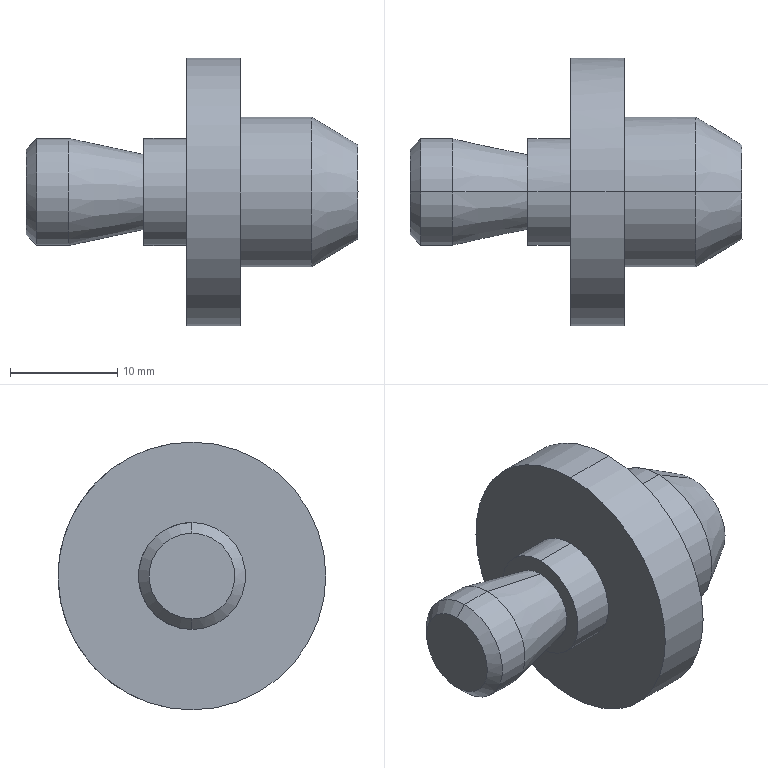Part | STEP file | Positioning_id1706_x_t | 1 solid | 19 faces | box 31 x 25 x 25 mm | volume 4946 mm3 | cylinder 8 | cone 6 | plane 5 | commonest cylinder face diameters 10 x4 14 x2 25 x2
STEP:
#1=CARTESIAN_POINT('',(0.,0.,0.));
#2=DIRECTION('',(0.,0.,1.));
#3=DIRECTION('',(1.,0.,0.));
#4=AXIS2_PLACEMENT_3D('',#1,#2,#3);
#5=CARTESIAN_POINT('',(-652.333,523.,129.997));
#6=VERTEX_POINT('',#5);
#7=CARTESIAN_POINT('',(-648.,523.,127.397));
#8=VERTEX_POINT('',#7);
#9=CARTESIAN_POINT('',(-648.,523.,127.397));
#10=DIRECTION('',(0.8575,0.,-0.5145));
#11=VECTOR('',#10,1.);
#12=LINE('',#9,#11);
#13=CARTESIAN_POINT('',(-654.,523.,122.997));
#14=DIRECTION('',(-1.,0.,0.));
#15=DIRECTION('',(0.,0.,1.));
#16=AXIS2_PLACEMENT_3D('',#13,#14,#15);
#17=CONICAL_SURFACE('',#16,8.,0.5404);
#18=CARTESIAN_POINT('',(0.,-6.));
#19=DIRECTION('',(0.,-1.));
#20=VECTOR('',#19,1.);
#21=LINE('',#18,#20);
#22=(GEOMETRIC_REPRESENTATION_CONTEXT(2)PARAMETRIC_REPRESENTATION_CONTEXT()REPRESENTATION_CONTEXT('',''));
#23=DEFINITIONAL_REPRESENTATION('',(#21),#22);
#24=PCURVE('',#17,#23);
#25=CARTESIAN_POINT('',(-654.,523.,122.997));
#26=DIRECTION('',(-1.,0.,0.));
#27=DIRECTION('',(0.,0.,1.));
#28=AXIS2_PLACEMENT_3D('',#25,#26,#27);
#29=CONICAL_SURFACE('',#28,8.,0.5404);
#30=CARTESIAN_POINT('',(6.283,-6.));
#31=DIRECTION('',(0.,-1.));
#32=VECTOR('',#31,1.);
#33=LINE('',#30,#32);
#34=(GEOMETRIC_REPRESENTATION_CONTEXT(2)PARAMETRIC_REPRESENTATION_CONTEXT()REPRESENTATION_CONTEXT('',''));
#35=DEFINITIONAL_REPRESENTATION('',(#33),#34);
#36=PCURVE('',#29,#35);
#37=SURFACE_CURVE('',#12,(#24,#36),.PCURVE_S1.);
#38=EDGE_CURVE('',#6,#8,#37,.T.);
#39=ORIENTED_EDGE('',*,*,#38,.T.);
#40=CARTESIAN_POINT('',(-648.,523.,118.597));
#41=VERTEX_POINT('',#40);
#42=CARTESIAN_POINT('',(-648.,523.,122.997));
#43=DIRECTION('',(-1.,0.,0.));
#44=DIRECTION('',(0.,0.,1.));
#45=AXIS2_PLACEMENT_3D('',#42,#43,#44);
#46=CIRCLE('',#45,4.4);
#47=CARTESIAN_POINT('',(0.,-6.));
#48=DIRECTION('',(1.,0.));
#49=VECTOR('',#48,1.);
#50=LINE('',#47,#49);
#51=(GEOMETRIC_REPRESENTATION_CONTEXT(2)PARAMETRIC_REPRESENTATION_CONTEXT()REPRESENTATION_CONTEXT('',''));
#52=DEFINITIONAL_REPRESENTATION('',(#50),#51);
#53=PCURVE('',#17,#52);
#54=CARTESIAN_POINT('',(-648.,523.,122.997));
#55=DIRECTION('',(1.,0.,0.));
#56=DIRECTION('',(0.,0.,1.));
#57=AXIS2_PLACEMENT_3D('',#54,#55,#56);
#58=PLANE('',#57);
#59=CARTESIAN_POINT('',(4.4,0.));
#60=CARTESIAN_POINT('',(4.4,-7.621));
#61=CARTESIAN_POINT('',(-2.2,-3.811));
#62=CARTESIAN_POINT('',(-8.8,0.));
#63=CARTESIAN_POINT('',(-2.2,3.811));
#64=CARTESIAN_POINT('',(4.4,7.621));
#65=CARTESIAN_POINT('',(4.4,0.));
#66=(BOUNDED_CURVE()B_SPLINE_CURVE(2,(#59,#60,#61,#62,#63,#64,#65),.UNSPECIFIED.,.T.,.F.)B_SPLINE_CURVE_WITH_KNOTS((1,2,2,2,2,1),(-2.094,0.,2.094,4.189,6.283,8.378),.UNSPECIFIED.)CURVE()GEOMETRIC_REPRESENTATION_ITEM()RATIONAL_B_SPLINE_CURVE((1.,0.5,1.,0.5,1.,0.5,1.))REPRESENTATION_ITEM(''));
#67=(GEOMETRIC_REPRESENTATION_CONTEXT(2)PARAMETRIC_REPRESENTATION_CONTEXT()REPRESENTATION_CONTEXT('',''));
#68=DEFINITIONAL_REPRESENTATION('',(#66),#67);
#69=PCURVE('',#58,#68);
#70=SURFACE_CURVE('',#46,(#53,#69),.PCURVE_S1.);
#71=EDGE_CURVE('',#8,#41,#70,.T.);
#72=ORIENTED_EDGE('',*,*,#71,.T.);
#73=CARTESIAN_POINT('',(-652.333,523.,115.997));
#74=VERTEX_POINT('',#73);
#75=CARTESIAN_POINT('',(-648.,523.,118.597));
#76=DIRECTION('',(-0.8575,0.,-0.5145));
#77=VECTOR('',#76,1.);
#78=LINE('',#75,#77);
#79=CARTESIAN_POINT('',(3.142,-6.));
#80=DIRECTION('',(0.,1.));
#81=VECTOR('',#80,1.);
#82=LINE('',#79,#81);
#83=(GEOMETRIC_REPRESENTATION_CONTEXT(2)PARAMETRIC_REPRESENTATION_CONTEXT()REPRESENTATION_CONTEXT('',''));
#84=DEFINITIONAL_REPRESENTATION('',(#82),#83);
#85=PCURVE('',#17,#84);
#86=CARTESIAN_POINT('',(3.142,-6.));
#87=DIRECTION('',(0.,1.));
#88=VECTOR('',#87,1.);
#89=LINE('',#86,#88);
#90=(GEOMETRIC_REPRESENTATION_CONTEXT(2)PARAMETRIC_REPRESENTATION_CONTEXT()REPRESENTATION_CONTEXT('',''));
#91=DEFINITIONAL_REPRESENTATION('',(#89),#90);
#92=PCURVE('',#29,#91);
#93=SURFACE_CURVE('',#78,(#85,#92),.PCURVE_S1.);
#94=EDGE_CURVE('',#41,#74,#93,.T.);
#95=ORIENTED_EDGE('',*,*,#94,.T.);
#96=CARTESIAN_POINT('',(-652.333,523.,122.997));
#97=DIRECTION('',(1.,0.,0.));
#98=DIRECTION('',(0.,0.,-1.));
#99=AXIS2_PLACEMENT_3D('',#96,#97,#98);
#100=CIRCLE('',#99,7.);
#101=CARTESIAN_POINT('',(3.142,-1.667));
#102=DIRECTION('',(-1.,0.));
#103=VECTOR('',#102,1.);
#104=LINE('',#101,#103);
#105=(GEOMETRIC_REPRESENTATION_CONTEXT(2)PARAMETRIC_REPRESENTATION_CONTEXT()REPRESENTATION_CONTEXT('',''));
#106=DEFINITIONAL_REPRESENTATION('',(#104),#105);
#107=PCURVE('',#17,#106);
#108=CARTESIAN_POINT('',(-659.,523.,122.997));
#109=DIRECTION('',(-1.,0.,0.));
#110=DIRECTION('',(0.,0.,1.));
#111=AXIS2_PLACEMENT_3D('',#108,#109,#110);
#112=CYLINDRICAL_SURFACE('',#111,7.);
#113=CARTESIAN_POINT('',(3.142,-6.667));
#114=DIRECTION('',(-1.,0.));
#115=VECTOR('',#114,1.);
#116=LINE('',#113,#115);
#117=(GEOMETRIC_REPRESENTATION_CONTEXT(2)PARAMETRIC_REPRESENTATION_CONTEXT()REPRESENTATION_CONTEXT('',''));
#118=DEFINITIONAL_REPRESENTATION('',(#116),#117);
#119=PCURVE('',#112,#118);
#120=SURFACE_CURVE('',#100,(#107,#119),.PCURVE_S1.);
#121=EDGE_CURVE('',#74,#6,#120,.T.);
#122=ORIENTED_EDGE('',*,*,#121,.T.);
#123=EDGE_LOOP('',(#39,#72,#95,#122));
#124=FACE_BOUND('',#123,.T.);
#125=ADVANCED_FACE('',(#124),#17,.T.);
#126=CARTESIAN_POINT('',(-659.,523.,129.997));
#127=VERTEX_POINT('',#126);
#128=CARTESIAN_POINT('',(-659.,523.,129.997));
#129=DIRECTION('',(1.,0.,0.));
#130=VECTOR('',#129,1.);
#131=LINE('',#128,#130);
#132=CARTESIAN_POINT('',(-659.,523.,122.997));
#133=DIRECTION('',(-1.,0.,0.));
#134=DIRECTION('',(0.,0.,1.));
#135=AXIS2_PLACEMENT_3D('',#132,#133,#134);
#136=CYLINDRICAL_SURFACE('',#135,7.);
#137=CARTESIAN_POINT('',(6.283,0.));
#138=DIRECTION('',(0.,-1.));
#139=VECTOR('',#138,1.);
#140=LINE('',#137,#139);
#141=(GEOMETRIC_REPRESENTATION_CONTEXT(2)PARAMETRIC_REPRESENTATION_CONTEXT()REPRESENTATION_CONTEXT('',''));
#142=DEFINITIONAL_REPRESENTATION('',(#140),#141);
#143=PCURVE('',#136,#142);
#144=CARTESIAN_POINT('',(0.,0.));
#145=DIRECTION('',(0.,-1.));
#146=VECTOR('',#145,1.);
#147=LINE('',#144,#146);
#148=(GEOMETRIC_REPRESENTATION_CONTEXT(2)PARAMETRIC_REPRESENTATION_CONTEXT()REPRESENTATION_CONTEXT('',''));
#149=DEFINITIONAL_REPRESENTATION('',(#147),#148);
#150=PCURVE('',#112,#149);
#151=SURFACE_CURVE('',#131,(#143,#150),.PCURVE_S1.);
#152=EDGE_CURVE('',#127,#6,#151,.T.);
#153=ORIENTED_EDGE('',*,*,#152,.F.);
#154=CARTESIAN_POINT('',(-659.,523.,115.997));
#155=VERTEX_POINT('',#154);
#156=CARTESIAN_POINT('',(-659.,523.,122.997));
#157=DIRECTION('',(-1.,0.,0.));
#158=DIRECTION('',(0.,0.,1.));
#159=AXIS2_PLACEMENT_3D('',#156,#157,#158);
#160=CIRCLE('',#159,7.);
#161=CARTESIAN_POINT('',(0.,0.));
#162=DIRECTION('',(1.,0.));
#163=VECTOR('',#162,1.);
#164=LINE('',#161,#163);
#165=(GEOMETRIC_REPRESENTATION_CONTEXT(2)PARAMETRIC_REPRESENTATION_CONTEXT()REPRESENTATION_CONTEXT('',''));
#166=DEFINITIONAL_REPRESENTATION('',(#164),#165);
#167=PCURVE('',#136,#166);
#168=CARTESIAN_POINT('',(-659.,523.,122.997));
#169=DIRECTION('',(1.,0.,0.));
#170=DIRECTION('',(0.,0.,1.));
#171=AXIS2_PLACEMENT_3D('',#168,#169,#170);
#172=PLANE('',#171);
#173=CARTESIAN_POINT('',(7.,0.));
#174=CARTESIAN_POINT('',(7.,-12.124));
#175=CARTESIAN_POINT('',(-3.5,-6.062));
#176=CARTESIAN_POINT('',(-14.,0.));
#177=CARTESIAN_POINT('',(-3.5,6.062));
#178=CARTESIAN_POINT('',(7.,12.124));
#179=CARTESIAN_POINT('',(7.,0.));
#180=(BOUNDED_CURVE()B_SPLINE_CURVE(2,(#173,#174,#175,#176,#177,#178,#179),.UNSPECIFIED.,.T.,.F.)B_SPLINE_CURVE_WITH_KNOTS((1,2,2,2,2,1),(-2.094,0.,2.094,4.189,6.283,8.378),.UNSPECIFIED.)CURVE()GEOMETRIC_REPRESENTATION_ITEM()RATIONAL_B_SPLINE_CURVE((1.,0.5,1.,0.5,1.,0.5,1.))REPRESENTATION_ITEM(''));
#181=(GEOMETRIC_REPRESENTATION_CONTEXT(2)PARAMETRIC_REPRESENTATION_CONTEXT()REPRESENTATION_CONTEXT('',''));
#182=DEFINITIONAL_REPRESENTATION('',(#180),#181);
#183=PCURVE('',#172,#182);
#184=SURFACE_CURVE('',#160,(#167,#183),.PCURVE_S1.);
#185=EDGE_CURVE('',#155,#127,#184,.T.);
#186=ORIENTED_EDGE('',*,*,#185,.F.);
#187=CARTESIAN_POINT('',(-659.,523.,115.997));
#188=DIRECTION('',(-1.,0.,0.));
#189=VECTOR('',#188,1.);
#190=LINE('',#187,#189);
#191=CARTESIAN_POINT('',(3.142,0.));
#192=DIRECTION('',(0.,1.));
#193=VECTOR('',#192,1.);
#194=LINE('',#191,#193);
#195=(GEOMETRIC_REPRESENTATION_CONTEXT(2)PARAMETRIC_REPRESENTATION_CONTEXT()REPRESENTATION_CONTEXT('',''));
#196=DEFINITIONAL_REPRESENTATION('',(#194),#195);
#197=PCURVE('',#136,#196);
#198=CARTESIAN_POINT('',(3.142,0.));
#199=DIRECTION('',(0.,1.));
#200=VECTOR('',#199,1.);
#201=LINE('',#198,#200);
#202=(GEOMETRIC_REPRESENTATION_CONTEXT(2)PARAMETRIC_REPRESENTATION_CONTEXT()REPRESENTATION_CONTEXT('',''));
#203=DEFINITIONAL_REPRESENTATION('',(#201),#202);
#204=PCURVE('',#112,#203);
#205=SURFACE_CURVE('',#190,(#197,#204),.PCURVE_S1.);
#206=EDGE_CURVE('',#74,#155,#205,.T.);
#207=ORIENTED_EDGE('',*,*,#206,.F.);
#208=CARTESIAN_POINT('',(-652.333,523.,122.997));
#209=DIRECTION('',(1.,0.,0.));
#210=DIRECTION('',(0.,0.,1.));
#211=AXIS2_PLACEMENT_3D('',#208,#209,#210);
#212=CIRCLE('',#211,7.);
#213=CARTESIAN_POINT('',(6.283,-6.667));
#214=DIRECTION('',(-1.,0.));
#215=VECTOR('',#214,1.);
#216=LINE('',#213,#215);
#217=(GEOMETRIC_REPRESENTATION_CONTEXT(2)PARAMETRIC_REPRESENTATION_CONTEXT()REPRESENTATION_CONTEXT('',''));
#218=DEFINITIONAL_REPRESENTATION('',(#216),#217);
#219=PCURVE('',#136,#218);
#220=CARTESIAN_POINT('',(6.283,-1.667));
#221=DIRECTION('',(-1.,0.));
#222=VECTOR('',#221,1.);
#223=LINE('',#220,#222);
#224=(GEOMETRIC_REPRESENTATION_CONTEXT(2)PARAMETRIC_REPRESENTATION_CONTEXT()REPRESENTATION_CONTEXT('',''));
#225=DEFINITIONAL_REPRESENTATION('',(#223),#224);
#226=PCURVE('',#29,#225);
#227=SURFACE_CURVE('',#212,(#219,#226),.PCURVE_S1.);
#228=EDGE_CURVE('',#6,#74,#227,.T.);
#229=ORIENTED_EDGE('',*,*,#228,.F.);
#230=EDGE_LOOP('',(#153,#186,#207,#229));
#231=FACE_BOUND('',#230,.T.);
#232=ADVANCED_FACE('',(#231),#136,.T.);
#233=CARTESIAN_POINT('',(-648.,523.,118.597));
#234=CARTESIAN_POINT('',(-648.,518.6,118.597));
#235=CARTESIAN_POINT('',(-648.,516.4,122.997));
#236=CARTESIAN_POINT('',(-648.,518.6,127.397));
#237=CARTESIAN_POINT('',(-648.,523.,127.397));
#238=(BOUNDED_CURVE()B_SPLINE_CURVE(4,(#233,#234,#235,#236,#237),.UNSPECIFIED.,.F.,.F.)B_SPLINE_CURVE_WITH_KNOTS((5,5),(0.,1.),.PIECEWISE_BEZIER_KNOTS.)CURVE()GEOMETRIC_REPRESENTATION_ITEM()RATIONAL_B_SPLINE_CURVE((1.,0.7071,0.6667,0.7071,1.))REPRESENTATION_ITEM(''));
#239=CARTESIAN_POINT('',(-4.4,0.));
#240=CARTESIAN_POINT('',(-4.4,4.4));
#241=CARTESIAN_POINT('',(0.,6.6));
#242=CARTESIAN_POINT('',(4.4,4.4));
#243=CARTESIAN_POINT('',(4.4,0.));
#244=(BOUNDED_CURVE()B_SPLINE_CURVE(4,(#239,#240,#241,#242,#243),.UNSPECIFIED.,.F.,.F.)B_SPLINE_CURVE_WITH_KNOTS((5,5),(0.,1.),.PIECEWISE_BEZIER_KNOTS.)CURVE()GEOMETRIC_REPRESENTATION_ITEM()RATIONAL_B_SPLINE_CURVE((1.,0.7071,0.6667,0.7071,1.))REPRESENTATION_ITEM(''));
#245=(GEOMETRIC_REPRESENTATION_CONTEXT(2)PARAMETRIC_REPRESENTATION_CONTEXT()REPRESENTATION_CONTEXT('',''));
#246=DEFINITIONAL_REPRESENTATION('',(#244),#245);
#247=PCURVE('',#58,#246);
#248=CARTESIAN_POINT('',(3.142,-6.));
#249=CARTESIAN_POINT('',(3.184,-6.));
#250=CARTESIAN_POINT('',(3.271,-6.));
#251=CARTESIAN_POINT('',(3.405,-6.));
#252=CARTESIAN_POINT('',(3.542,-6.));
#253=CARTESIAN_POINT('',(3.681,-6.));
#254=CARTESIAN_POINT('',(3.823,-6.));
#255=CARTESIAN_POINT('',(3.968,-6.));
#256=CARTESIAN_POINT('',(4.114,-6.));
#257=CARTESIAN_POINT('',(4.262,-6.));
#258=CARTESIAN_POINT('',(4.412,-6.));
#259=CARTESIAN_POINT('',(4.562,-6.));
#260=CARTESIAN_POINT('',(4.712,-6.));
#261=CARTESIAN_POINT('',(4.863,-6.));
#262=CARTESIAN_POINT('',(5.013,-6.));
#263=CARTESIAN_POINT('',(5.163,-6.));
#264=CARTESIAN_POINT('',(5.311,-6.));
#265=CARTESIAN_POINT('',(5.457,-6.));
#266=CARTESIAN_POINT('',(5.602,-6.));
#267=CARTESIAN_POINT('',(5.744,-6.));
#268=CARTESIAN_POINT('',(5.883,-6.));
#269=CARTESIAN_POINT('',(6.02,-6.));
#270=CARTESIAN_POINT('',(6.153,-6.));
#271=CARTESIAN_POINT('',(6.24,-6.));
#272=CARTESIAN_POINT('',(6.283,-6.));
#273=B_SPLINE_CURVE_WITH_KNOTS('',3,(#248,#249,#250,#251,#252,#253,#254,#255,#256,#257,#258,#259,#260,#261,#262,#263,#264,#265,#266,#267,#268,#269,#270,#271,#272),.UNSPECIFIED.,.F.,.F.,(4,1,1,1,1,1,1,1,1,1,1,1,1,1,1,1,1,1,1,1,1,1,4),(0.,0.04545,0.09091,0.1364,0.1818,0.2273,0.2727,0.3182,0.3636,0.4091,0.4545,0.5,0.5455,0.5909,0.6364,0.6818,0.7273,0.7727,0.8182,0.8636,0.9091,0.9545,1.),.QUASI_UNIFORM_KNOTS.);
#274=(GEOMETRIC_REPRESENTATION_CONTEXT(2)PARAMETRIC_REPRESENTATION_CONTEXT()REPRESENTATION_CONTEXT('',''));
#275=DEFINITIONAL_REPRESENTATION('',(#273),#274);
#276=PCURVE('',#29,#275);
#277=SURFACE_CURVE('',#238,(#247,#276),.PCURVE_S1.);
#278=EDGE_CURVE('',#41,#8,#277,.T.);
#279=ORIENTED_EDGE('',*,*,#278,.F.);
#280=ORIENTED_EDGE('',*,*,#71,.F.);
#281=EDGE_LOOP('',(#279,#280));
#282=FACE_BOUND('',#281,.T.);
#283=ADVANCED_FACE('',(#282),#58,.T.);
#284=CARTESIAN_POINT('',(-668.,523.,119.497));
#285=VERTEX_POINT('',#284);
#286=CARTESIAN_POINT('',(-668.,523.,126.497));
#287=VERTEX_POINT('',#286);
#288=CARTESIAN_POINT('',(-668.,523.,122.997));
#289=DIRECTION('',(-1.,0.,0.));
#290=DIRECTION('',(0.,0.,-1.));
#291=AXIS2_PLACEMENT_3D('',#288,#289,#290);
#292=CIRCLE('',#291,3.5);
#293=CARTESIAN_POINT('',(-668.,523.,122.997));
#294=DIRECTION('',(1.,0.,0.));
#295=DIRECTION('',(0.,0.,1.));
#296=AXIS2_PLACEMENT_3D('',#293,#294,#295);
#297=PLANE('',#296);
#298=CARTESIAN_POINT('',(-3.5,0.));
#299=CARTESIAN_POINT('',(-3.5,6.062));
#300=CARTESIAN_POINT('',(1.75,3.031));
#301=CARTESIAN_POINT('',(7.,0.));
#302=CARTESIAN_POINT('',(1.75,-3.031));
#303=CARTESIAN_POINT('',(-3.5,-6.062));
#304=CARTESIAN_POINT('',(-3.5,0.));
#305=(BOUNDED_CURVE()B_SPLINE_CURVE(2,(#298,#299,#300,#301,#302,#303,#304),.UNSPECIFIED.,.T.,.F.)B_SPLINE_CURVE_WITH_KNOTS((1,2,2,2,2,1),(-2.094,0.,2.094,4.189,6.283,8.378),.UNSPECIFIED.)CURVE()GEOMETRIC_REPRESENTATION_ITEM()RATIONAL_B_SPLINE_CURVE((1.,0.5,1.,0.5,1.,0.5,1.))REPRESENTATION_ITEM(''));
#306=(GEOMETRIC_REPRESENTATION_CONTEXT(2)PARAMETRIC_REPRESENTATION_CONTEXT()REPRESENTATION_CONTEXT('',''));
#307=DEFINITIONAL_REPRESENTATION('',(#305),#306);
#308=PCURVE('',#297,#307);
#309=CARTESIAN_POINT('',(-675.,523.,122.997));
#310=DIRECTION('',(-1.,0.,0.));
#311=DIRECTION('',(0.,0.,1.));
#312=AXIS2_PLACEMENT_3D('',#309,#310,#311);
#313=CONICAL_SURFACE('',#312,5.,0.2111);
#314=CARTESIAN_POINT('',(3.142,-7.));
#315=DIRECTION('',(1.,0.));
#316=VECTOR('',#315,1.);
#317=LINE('',#314,#316);
#318=(GEOMETRIC_REPRESENTATION_CONTEXT(2)PARAMETRIC_REPRESENTATION_CONTEXT()REPRESENTATION_CONTEXT('',''));
#319=DEFINITIONAL_REPRESENTATION('',(#317),#318);
#320=PCURVE('',#313,#319);
#321=SURFACE_CURVE('',#292,(#308,#320),.PCURVE_S1.);
#322=EDGE_CURVE('',#285,#287,#321,.T.);
#323=ORIENTED_EDGE('',*,*,#322,.F.);
#324=CARTESIAN_POINT('',(-668.,523.,122.997));
#325=DIRECTION('',(-1.,0.,0.));
#326=DIRECTION('',(0.,0.,1.));
#327=AXIS2_PLACEMENT_3D('',#324,#325,#326);
#328=CIRCLE('',#327,3.5);
#329=CARTESIAN_POINT('',(3.5,0.));
#330=CARTESIAN_POINT('',(3.5,-6.062));
#331=CARTESIAN_POINT('',(-1.75,-3.031));
#332=CARTESIAN_POINT('',(-7.,0.));
#333=CARTESIAN_POINT('',(-1.75,3.031));
#334=CARTESIAN_POINT('',(3.5,6.062));
#335=CARTESIAN_POINT('',(3.5,0.));
#336=(BOUNDED_CURVE()B_SPLINE_CURVE(2,(#329,#330,#331,#332,#333,#334,#335),.UNSPECIFIED.,.T.,.F.)B_SPLINE_CURVE_WITH_KNOTS((1,2,2,2,2,1),(-2.094,0.,2.094,4.189,6.283,8.378),.UNSPECIFIED.)CURVE()GEOMETRIC_REPRESENTATION_ITEM()RATIONAL_B_SPLINE_CURVE((1.,0.5,1.,0.5,1.,0.5,1.))REPRESENTATION_ITEM(''));
#337=(GEOMETRIC_REPRESENTATION_CONTEXT(2)PARAMETRIC_REPRESENTATION_CONTEXT()REPRESENTATION_CONTEXT('',''));
#338=DEFINITIONAL_REPRESENTATION('',(#336),#337);
#339=PCURVE('',#297,#338);
#340=CARTESIAN_POINT('',(-675.,523.,122.997));
#341=DIRECTION('',(-1.,0.,0.));
#342=DIRECTION('',(0.,0.,1.));
#343=AXIS2_PLACEMENT_3D('',#340,#341,#342);
#344=CONICAL_SURFACE('',#343,5.,0.2111);
#345=CARTESIAN_POINT('',(0.,-7.));
#346=DIRECTION('',(1.,0.));
#347=VECTOR('',#346,1.);
#348=LINE('',#345,#347);
#349=(GEOMETRIC_REPRESENTATION_CONTEXT(2)PARAMETRIC_REPRESENTATION_CONTEXT()REPRESENTATION_CONTEXT('',''));
#350=DEFINITIONAL_REPRESENTATION('',(#348),#349);
#351=PCURVE('',#344,#350);
#352=SURFACE_CURVE('',#328,(#339,#351),.PCURVE_S1.);
#353=EDGE_CURVE('',#287,#285,#352,.T.);
#354=ORIENTED_EDGE('',*,*,#353,.F.);
#355=EDGE_LOOP('',(#323,#354));
#356=FACE_BOUND('',#355,.T.);
#357=CARTESIAN_POINT('',(-668.,523.,117.997));
#358=VERTEX_POINT('',#357);
#359=CARTESIAN_POINT('',(-668.,523.,127.997));
#360=VERTEX_POINT('',#359);
#361=CARTESIAN_POINT('',(-668.,523.,122.997));
#362=DIRECTION('',(1.,0.,0.));
#363=DIRECTION('',(0.,0.,-1.));
#364=AXIS2_PLACEMENT_3D('',#361,#362,#363);
#365=CIRCLE('',#364,5.);
#366=CARTESIAN_POINT('',(0.,0.));
#367=DIRECTION('',(-1.,0.));
#368=AXIS2_PLACEMENT_2D('',#366,#367);
#369=CIRCLE('',#368,5.);
#370=(GEOMETRIC_REPRESENTATION_CONTEXT(2)PARAMETRIC_REPRESENTATION_CONTEXT()REPRESENTATION_CONTEXT('',''));
#371=DEFINITIONAL_REPRESENTATION('',(#369),#370);
#372=PCURVE('',#297,#371);
#373=CARTESIAN_POINT('',(-669.,523.,122.997));
#374=DIRECTION('',(-1.,0.,0.));
#375=DIRECTION('',(0.,0.,1.));
#376=AXIS2_PLACEMENT_3D('',#373,#374,#375);
#377=CYLINDRICAL_SURFACE('',#376,5.);
#378=CARTESIAN_POINT('',(3.142,-1.));
#379=DIRECTION('',(-1.,0.));
#380=VECTOR('',#379,1.);
#381=LINE('',#378,#380);
#382=(GEOMETRIC_REPRESENTATION_CONTEXT(2)PARAMETRIC_REPRESENTATION_CONTEXT()REPRESENTATION_CONTEXT('',''));
#383=DEFINITIONAL_REPRESENTATION('',(#381),#382);
#384=PCURVE('',#377,#383);
#385=SURFACE_CURVE('',#365,(#372,#384),.PCURVE_S1.);
#386=EDGE_CURVE('',#358,#360,#385,.T.);
#387=ORIENTED_EDGE('',*,*,#386,.F.);
#388=CARTESIAN_POINT('',(-668.,523.,122.997));
#389=DIRECTION('',(1.,0.,0.));
#390=DIRECTION('',(0.,0.,1.));
#391=AXIS2_PLACEMENT_3D('',#388,#389,#390);
#392=CIRCLE('',#391,5.);
#393=CARTESIAN_POINT('',(0.,0.));
#394=DIRECTION('',(1.,0.));
#395=AXIS2_PLACEMENT_2D('',#393,#394);
#396=CIRCLE('',#395,5.);
#397=(GEOMETRIC_REPRESENTATION_CONTEXT(2)PARAMETRIC_REPRESENTATION_CONTEXT()REPRESENTATION_CONTEXT('',''));
#398=DEFINITIONAL_REPRESENTATION('',(#396),#397);
#399=PCURVE('',#297,#398);
#400=CARTESIAN_POINT('',(-669.,523.,122.997));
#401=DIRECTION('',(-1.,0.,0.));
#402=DIRECTION('',(0.,0.,1.));
#403=AXIS2_PLACEMENT_3D('',#400,#401,#402);
#404=CYLINDRICAL_SURFACE('',#403,5.);
#405=CARTESIAN_POINT('',(6.283,-1.));
#406=DIRECTION('',(-1.,0.));
#407=VECTOR('',#406,1.);
#408=LINE('',#405,#407);
#409=(GEOMETRIC_REPRESENTATION_CONTEXT(2)PARAMETRIC_REPRESENTATION_CONTEXT()REPRESENTATION_CONTEXT('',''));
#410=DEFINITIONAL_REPRESENTATION('',(#408),#409);
#411=PCURVE('',#404,#410);
#412=SURFACE_CURVE('',#392,(#399,#411),.PCURVE_S1.);
#413=EDGE_CURVE('',#360,#358,#412,.T.);
#414=ORIENTED_EDGE('',*,*,#413,.F.);
#415=EDGE_LOOP('',(#387,#414));
#416=FACE_BOUND('',#415,.T.);
#417=ADVANCED_FACE('',(#356,#416),#297,.F.);
#418=CARTESIAN_POINT('',(-664.,523.,127.997));
#419=VERTEX_POINT('',#418);
#420=CARTESIAN_POINT('',(-668.,523.,127.997));
#421=DIRECTION('',(1.,0.,0.));
#422=VECTOR('',#421,1.);
#423=LINE('',#420,#422);
#424=CARTESIAN_POINT('',(6.283,-1.));
#425=DIRECTION('',(0.,-1.));
#426=VECTOR('',#425,1.);
#427=LINE('',#424,#426);
#428=(GEOMETRIC_REPRESENTATION_CONTEXT(2)PARAMETRIC_REPRESENTATION_CONTEXT()REPRESENTATION_CONTEXT('',''));
#429=DEFINITIONAL_REPRESENTATION('',(#427),#428);
#430=PCURVE('',#404,#429);
#431=CARTESIAN_POINT('',(0.,-1.));
#432=DIRECTION('',(0.,-1.));
#433=VECTOR('',#432,1.);
#434=LINE('',#431,#433);
#435=(GEOMETRIC_REPRESENTATION_CONTEXT(2)PARAMETRIC_REPRESENTATION_CONTEXT()REPRESENTATION_CONTEXT('',''));
#436=DEFINITIONAL_REPRESENTATION('',(#434),#435);
#437=PCURVE('',#377,#436);
#438=SURFACE_CURVE('',#423,(#430,#437),.PCURVE_S1.);
#439=EDGE_CURVE('',#360,#419,#438,.T.);
#440=ORIENTED_EDGE('',*,*,#439,.F.);
#441=ORIENTED_EDGE('',*,*,#413,.T.);
#442=CARTESIAN_POINT('',(-664.,523.,117.997));
#443=VERTEX_POINT('',#442);
#444=CARTESIAN_POINT('',(-668.,523.,117.997));
#445=DIRECTION('',(-1.,0.,0.));
#446=VECTOR('',#445,1.);
#447=LINE('',#444,#446);
#448=CARTESIAN_POINT('',(3.142,-1.));
#449=DIRECTION('',(0.,1.));
#450=VECTOR('',#449,1.);
#451=LINE('',#448,#450);
#452=(GEOMETRIC_REPRESENTATION_CONTEXT(2)PARAMETRIC_REPRESENTATION_CONTEXT()REPRESENTATION_CONTEXT('',''));
#453=DEFINITIONAL_REPRESENTATION('',(#451),#452);
#454=PCURVE('',#404,#453);
#455=CARTESIAN_POINT('',(3.142,-1.));
#456=DIRECTION('',(0.,1.));
#457=VECTOR('',#456,1.);
#458=LINE('',#455,#457);
#459=(GEOMETRIC_REPRESENTATION_CONTEXT(2)PARAMETRIC_REPRESENTATION_CONTEXT()REPRESENTATION_CONTEXT('',''));
#460=DEFINITIONAL_REPRESENTATION('',(#458),#459);
#461=PCURVE('',#377,#460);
#462=SURFACE_CURVE('',#447,(#454,#461),.PCURVE_S1.);
#463=EDGE_CURVE('',#443,#358,#462,.T.);
#464=ORIENTED_EDGE('',*,*,#463,.F.);
#465=CARTESIAN_POINT('',(-664.,523.,122.997));
#466=DIRECTION('',(1.,0.,0.));
#467=DIRECTION('',(0.,0.,1.));
#468=AXIS2_PLACEMENT_3D('',#465,#466,#467);
#469=CIRCLE('',#468,5.);
#470=CARTESIAN_POINT('',(6.283,-5.));
#471=DIRECTION('',(-1.,0.));
#472=VECTOR('',#471,1.);
#473=LINE('',#470,#472);
#474=(GEOMETRIC_REPRESENTATION_CONTEXT(2)PARAMETRIC_REPRESENTATION_CONTEXT()REPRESENTATION_CONTEXT('',''));
#475=DEFINITIONAL_REPRESENTATION('',(#473),#474);
#476=PCURVE('',#404,#475);
#477=CARTESIAN_POINT('',(-664.,523.,122.997));
#478=DIRECTION('',(-1.,0.,0.));
#479=DIRECTION('',(0.,0.,-1.));
#480=AXIS2_PLACEMENT_3D('',#477,#478,#479);
#481=PLANE('',#480);
#482=CARTESIAN_POINT('',(-5.,0.));
#483=CARTESIAN_POINT('',(-5.,8.66));
#484=CARTESIAN_POINT('',(2.5,4.33));
#485=CARTESIAN_POINT('',(10.,0.));
#486=CARTESIAN_POINT('',(2.5,-4.33));
#487=CARTESIAN_POINT('',(-5.,-8.66));
#488=CARTESIAN_POINT('',(-5.,0.));
#489=(BOUNDED_CURVE()B_SPLINE_CURVE(2,(#482,#483,#484,#485,#486,#487,#488),.UNSPECIFIED.,.T.,.F.)B_SPLINE_CURVE_WITH_KNOTS((1,2,2,2,2,1),(-2.094,0.,2.094,4.189,6.283,8.378),.UNSPECIFIED.)CURVE()GEOMETRIC_REPRESENTATION_ITEM()RATIONAL_B_SPLINE_CURVE((1.,0.5,1.,0.5,1.,0.5,1.))REPRESENTATION_ITEM(''));
#490=(GEOMETRIC_REPRESENTATION_CONTEXT(2)PARAMETRIC_REPRESENTATION_CONTEXT()REPRESENTATION_CONTEXT('',''));
#491=DEFINITIONAL_REPRESENTATION('',(#489),#490);
#492=PCURVE('',#481,#491);
#493=SURFACE_CURVE('',#469,(#476,#492),.PCURVE_S1.);
#494=EDGE_CURVE('',#419,#443,#493,.T.);
#495=ORIENTED_EDGE('',*,*,#494,.F.);
#496=EDGE_LOOP('',(#440,#441,#464,#495));
#497=FACE_BOUND('',#496,.T.);
#498=ADVANCED_FACE('',(#497),#404,.T.);
#499=CARTESIAN_POINT('',(-675.,523.,127.997));
#500=VERTEX_POINT('',#499);
#501=CARTESIAN_POINT('',(-668.,523.,126.497));
#502=DIRECTION('',(0.9778,0.,-0.2095));
#503=VECTOR('',#502,1.);
#504=LINE('',#501,#503);
#505=CARTESIAN_POINT('',(0.,-7.));
#506=DIRECTION('',(0.,-1.));
#507=VECTOR('',#506,1.);
#508=LINE('',#505,#507);
#509=(GEOMETRIC_REPRESENTATION_CONTEXT(2)PARAMETRIC_REPRESENTATION_CONTEXT()REPRESENTATION_CONTEXT('',''));
#510=DEFINITIONAL_REPRESENTATION('',(#508),#509);
#511=PCURVE('',#344,#510);
#512=CARTESIAN_POINT('',(6.283,-7.));
#513=DIRECTION('',(0.,-1.));
#514=VECTOR('',#513,1.);
#515=LINE('',#512,#514);
#516=(GEOMETRIC_REPRESENTATION_CONTEXT(2)PARAMETRIC_REPRESENTATION_CONTEXT()REPRESENTATION_CONTEXT('',''));
#517=DEFINITIONAL_REPRESENTATION('',(#515),#516);
#518=PCURVE('',#313,#517);
#519=SURFACE_CURVE('',#504,(#511,#518),.PCURVE_S1.);
#520=EDGE_CURVE('',#500,#287,#519,.T.);
#521=ORIENTED_EDGE('',*,*,#520,.T.);
#522=ORIENTED_EDGE('',*,*,#353,.T.);
#523=CARTESIAN_POINT('',(-675.,523.,117.997));
#524=VERTEX_POINT('',#523);
#525=CARTESIAN_POINT('',(-668.,523.,119.497));
#526=DIRECTION('',(-0.9778,0.,-0.2095));
#527=VECTOR('',#526,1.);
#528=LINE('',#525,#527);
#529=CARTESIAN_POINT('',(3.142,-7.));
#530=DIRECTION('',(0.,1.));
#531=VECTOR('',#530,1.);
#532=LINE('',#529,#531);
#533=(GEOMETRIC_REPRESENTATION_CONTEXT(2)PARAMETRIC_REPRESENTATION_CONTEXT()REPRESENTATION_CONTEXT('',''));
#534=DEFINITIONAL_REPRESENTATION('',(#532),#533);
#535=PCURVE('',#344,#534);
#536=CARTESIAN_POINT('',(3.142,-7.));
#537=DIRECTION('',(0.,1.));
#538=VECTOR('',#537,1.);
#539=LINE('',#536,#538);
#540=(GEOMETRIC_REPRESENTATION_CONTEXT(2)PARAMETRIC_REPRESENTATION_CONTEXT()REPRESENTATION_CONTEXT('',''));
#541=DEFINITIONAL_REPRESENTATION('',(#539),#540);
#542=PCURVE('',#313,#541);
#543=SURFACE_CURVE('',#528,(#535,#542),.PCURVE_S1.);
#544=EDGE_CURVE('',#285,#524,#543,.T.);
#545=ORIENTED_EDGE('',*,*,#544,.T.);
#546=CARTESIAN_POINT('',(-675.,523.,122.997));
#547=DIRECTION('',(1.,0.,0.));
#548=DIRECTION('',(0.,0.,-1.));
#549=AXIS2_PLACEMENT_3D('',#546,#547,#548);
#550=CIRCLE('',#549,5.);
#551=CARTESIAN_POINT('',(3.142,0.));
#552=DIRECTION('',(-1.,0.));
#553=VECTOR('',#552,1.);
#554=LINE('',#551,#553);
#555=(GEOMETRIC_REPRESENTATION_CONTEXT(2)PARAMETRIC_REPRESENTATION_CONTEXT()REPRESENTATION_CONTEXT('',''));
#556=DEFINITIONAL_REPRESENTATION('',(#554),#555);
#557=PCURVE('',#344,#556);
#558=CARTESIAN_POINT('',(-669.,523.,122.997));
#559=DIRECTION('',(-1.,0.,0.));
#560=DIRECTION('',(0.,0.,1.));
#561=AXIS2_PLACEMENT_3D('',#558,#559,#560);
#562=CYLINDRICAL_SURFACE('',#561,5.);
#563=CARTESIAN_POINT('',(3.142,6.));
#564=DIRECTION('',(-1.,0.));
#565=VECTOR('',#564,1.);
#566=LINE('',#563,#565);
#567=(GEOMETRIC_REPRESENTATION_CONTEXT(2)PARAMETRIC_REPRESENTATION_CONTEXT()REPRESENTATION_CONTEXT('',''));
#568=DEFINITIONAL_REPRESENTATION('',(#566),#567);
#569=PCURVE('',#562,#568);
#570=SURFACE_CURVE('',#550,(#557,#569),.PCURVE_S1.);
#571=EDGE_CURVE('',#524,#500,#570,.T.);
#572=ORIENTED_EDGE('',*,*,#571,.T.);
#573=EDGE_LOOP('',(#521,#522,#545,#572));
#574=FACE_BOUND('',#573,.T.);
#575=ADVANCED_FACE('',(#574),#344,.T.);
#576=CARTESIAN_POINT('',(-678.,523.,117.997));
#577=VERTEX_POINT('',#576);
#578=CARTESIAN_POINT('',(-679.,523.,118.997));
#579=VERTEX_POINT('',#578);
#580=CARTESIAN_POINT('',(-679.,523.,118.997));
#581=DIRECTION('',(-0.7071,0.,0.7071));
#582=VECTOR('',#581,1.);
#583=LINE('',#580,#582);
#584=CARTESIAN_POINT('',(-678.,523.,122.997));
#585=DIRECTION('',(1.,0.,0.));
#586=DIRECTION('',(0.,0.,-1.));
#587=AXIS2_PLACEMENT_3D('',#584,#585,#586);
#588=CONICAL_SURFACE('',#587,5.,0.7854);
#589=CARTESIAN_POINT('',(0.,-1.));
#590=DIRECTION('',(0.,-1.));
#591=VECTOR('',#590,1.);
#592=LINE('',#589,#591);
#593=(GEOMETRIC_REPRESENTATION_CONTEXT(2)PARAMETRIC_REPRESENTATION_CONTEXT()REPRESENTATION_CONTEXT('',''));
#594=DEFINITIONAL_REPRESENTATION('',(#592),#593);
#595=PCURVE('',#588,#594);
#596=CARTESIAN_POINT('',(-678.,523.,122.997));
#597=DIRECTION('',(1.,0.,0.));
#598=DIRECTION('',(0.,0.,-1.));
#599=AXIS2_PLACEMENT_3D('',#596,#597,#598);
#600=CONICAL_SURFACE('',#599,5.,0.7854);
#601=CARTESIAN_POINT('',(6.283,-1.));
#602=DIRECTION('',(0.,-1.));
#603=VECTOR('',#602,1.);
#604=LINE('',#601,#603);
#605=(GEOMETRIC_REPRESENTATION_CONTEXT(2)PARAMETRIC_REPRESENTATION_CONTEXT()REPRESENTATION_CONTEXT('',''));
#606=DEFINITIONAL_REPRESENTATION('',(#604),#605);
#607=PCURVE('',#600,#606);
#608=SURFACE_CURVE('',#583,(#595,#607),.PCURVE_S1.);
#609=EDGE_CURVE('',#577,#579,#608,.T.);
#610=ORIENTED_EDGE('',*,*,#609,.T.);
#611=CARTESIAN_POINT('',(-679.,523.,126.997));
#612=VERTEX_POINT('',#611);
#613=CARTESIAN_POINT('',(-679.,523.,122.997));
#614=DIRECTION('',(1.,0.,0.));
#615=DIRECTION('',(0.,0.,-1.));
#616=AXIS2_PLACEMENT_3D('',#613,#614,#615);
#617=CIRCLE('',#616,4.);
#618=CARTESIAN_POINT('',(0.,-1.));
#619=DIRECTION('',(1.,0.));
#620=VECTOR('',#619,1.);
#621=LINE('',#618,#620);
#622=(GEOMETRIC_REPRESENTATION_CONTEXT(2)PARAMETRIC_REPRESENTATION_CONTEXT()REPRESENTATION_CONTEXT('',''));
#623=DEFINITIONAL_REPRESENTATION('',(#621),#622);
#624=PCURVE('',#588,#623);
#625=CARTESIAN_POINT('',(-679.,523.,122.997));
#626=DIRECTION('',(-1.,0.,0.));
#627=DIRECTION('',(0.,0.,-1.));
#628=AXIS2_PLACEMENT_3D('',#625,#626,#627);
#629=PLANE('',#628);
#630=CARTESIAN_POINT('',(4.,0.));
#631=CARTESIAN_POINT('',(4.,-6.928));
#632=CARTESIAN_POINT('',(-2.,-3.464));
#633=CARTESIAN_POINT('',(-8.,0.));
#634=CARTESIAN_POINT('',(-2.,3.464));
#635=CARTESIAN_POINT('',(4.,6.928));
#636=CARTESIAN_POINT('',(4.,0.));
#637=(BOUNDED_CURVE()B_SPLINE_CURVE(2,(#630,#631,#632,#633,#634,#635,#636),.UNSPECIFIED.,.T.,.F.)B_SPLINE_CURVE_WITH_KNOTS((1,2,2,2,2,1),(-2.094,0.,2.094,4.189,6.283,8.378),.UNSPECIFIED.)CURVE()GEOMETRIC_REPRESENTATION_ITEM()RATIONAL_B_SPLINE_CURVE((1.,0.5,1.,0.5,1.,0.5,1.))REPRESENTATION_ITEM(''));
#638=(GEOMETRIC_REPRESENTATION_CONTEXT(2)PARAMETRIC_REPRESENTATION_CONTEXT()REPRESENTATION_CONTEXT('',''));
#639=DEFINITIONAL_REPRESENTATION('',(#637),#638);
#640=PCURVE('',#629,#639);
#641=SURFACE_CURVE('',#617,(#624,#640),.PCURVE_S1.);
#642=EDGE_CURVE('',#579,#612,#641,.T.);
#643=ORIENTED_EDGE('',*,*,#642,.T.);
#644=CARTESIAN_POINT('',(-678.,523.,127.997));
#645=VERTEX_POINT('',#644);
#646=CARTESIAN_POINT('',(-679.,523.,126.997));
#647=DIRECTION('',(0.7071,0.,0.7071));
#648=VECTOR('',#647,1.);
#649=LINE('',#646,#648);
#650=CARTESIAN_POINT('',(3.142,-1.));
#651=DIRECTION('',(0.,1.));
#652=VECTOR('',#651,1.);
#653=LINE('',#650,#652);
#654=(GEOMETRIC_REPRESENTATION_CONTEXT(2)PARAMETRIC_REPRESENTATION_CONTEXT()REPRESENTATION_CONTEXT('',''));
#655=DEFINITIONAL_REPRESENTATION('',(#653),#654);
#656=PCURVE('',#588,#655);
#657=CARTESIAN_POINT('',(3.142,-1.));
#658=DIRECTION('',(0.,1.));
#659=VECTOR('',#658,1.);
#660=LINE('',#657,#659);
#661=(GEOMETRIC_REPRESENTATION_CONTEXT(2)PARAMETRIC_REPRESENTATION_CONTEXT()REPRESENTATION_CONTEXT('',''));
#662=DEFINITIONAL_REPRESENTATION('',(#660),#661);
#663=PCURVE('',#600,#662);
#664=SURFACE_CURVE('',#649,(#656,#663),.PCURVE_S1.);
#665=EDGE_CURVE('',#612,#645,#664,.T.);
#666=ORIENTED_EDGE('',*,*,#665,.T.);
#667=CARTESIAN_POINT('',(-678.,523.,122.997));
#668=DIRECTION('',(-1.,0.,0.));
#669=DIRECTION('',(0.,0.,1.));
#670=AXIS2_PLACEMENT_3D('',#667,#668,#669);
#671=CIRCLE('',#670,5.);
#672=CARTESIAN_POINT('',(3.142,0.));
#673=DIRECTION('',(-1.,0.));
#674=VECTOR('',#673,1.);
#675=LINE('',#672,#674);
#676=(GEOMETRIC_REPRESENTATION_CONTEXT(2)PARAMETRIC_REPRESENTATION_CONTEXT()REPRESENTATION_CONTEXT('',''));
#677=DEFINITIONAL_REPRESENTATION('',(#675),#676);
#678=PCURVE('',#588,#677);
#679=CARTESIAN_POINT('',(0.,9.));
#680=DIRECTION('',(1.,0.));
#681=VECTOR('',#680,1.);
#682=LINE('',#679,#681);
#683=(GEOMETRIC_REPRESENTATION_CONTEXT(2)PARAMETRIC_REPRESENTATION_CONTEXT()REPRESENTATION_CONTEXT('',''));
#684=DEFINITIONAL_REPRESENTATION('',(#682),#683);
#685=PCURVE('',#562,#684);
#686=SURFACE_CURVE('',#671,(#678,#685),.PCURVE_S1.);
#687=EDGE_CURVE('',#645,#577,#686,.T.);
#688=ORIENTED_EDGE('',*,*,#687,.T.);
#689=EDGE_LOOP('',(#610,#643,#666,#688));
#690=FACE_BOUND('',#689,.T.);
#691=ADVANCED_FACE('',(#690),#588,.T.);
#692=CARTESIAN_POINT('',(-678.,523.,127.997));
#693=DIRECTION('',(1.,0.,0.));
#694=VECTOR('',#693,1.);
#695=LINE('',#692,#694);
#696=CARTESIAN_POINT('',(-669.,523.,122.997));
#697=DIRECTION('',(-1.,0.,0.));
#698=DIRECTION('',(0.,0.,1.));
#699=AXIS2_PLACEMENT_3D('',#696,#697,#698);
#700=CYLINDRICAL_SURFACE('',#699,5.);
#701=CARTESIAN_POINT('',(6.283,9.));
#702=DIRECTION('',(0.,-1.));
#703=VECTOR('',#702,1.);
#704=LINE('',#701,#703);
#705=(GEOMETRIC_REPRESENTATION_CONTEXT(2)PARAMETRIC_REPRESENTATION_CONTEXT()REPRESENTATION_CONTEXT('',''));
#706=DEFINITIONAL_REPRESENTATION('',(#704),#705);
#707=PCURVE('',#700,#706);
#708=CARTESIAN_POINT('',(0.,9.));
#709=DIRECTION('',(0.,-1.));
#710=VECTOR('',#709,1.);
#711=LINE('',#708,#710);
#712=(GEOMETRIC_REPRESENTATION_CONTEXT(2)PARAMETRIC_REPRESENTATION_CONTEXT()REPRESENTATION_CONTEXT('',''));
#713=DEFINITIONAL_REPRESENTATION('',(#711),#712);
#714=PCURVE('',#562,#713);
#715=SURFACE_CURVE('',#695,(#707,#714),.PCURVE_S1.);
#716=EDGE_CURVE('',#645,#500,#715,.T.);
#717=ORIENTED_EDGE('',*,*,#716,.F.);
#718=CARTESIAN_POINT('',(-678.,523.,122.997));
#719=DIRECTION('',(-1.,0.,0.));
#720=DIRECTION('',(0.,0.,-1.));
#721=AXIS2_PLACEMENT_3D('',#718,#719,#720);
#722=CIRCLE('',#721,5.);
#723=CARTESIAN_POINT('',(3.142,9.));
#724=DIRECTION('',(1.,0.));
#725=VECTOR('',#724,1.);
#726=LINE('',#723,#725);
#727=(GEOMETRIC_REPRESENTATION_CONTEXT(2)PARAMETRIC_REPRESENTATION_CONTEXT()REPRESENTATION_CONTEXT('',''));
#728=DEFINITIONAL_REPRESENTATION('',(#726),#727);
#729=PCURVE('',#700,#728);
#730=CARTESIAN_POINT('',(6.283,0.));
#731=DIRECTION('',(-1.,0.));
#732=VECTOR('',#731,1.);
#733=LINE('',#730,#732);
#734=(GEOMETRIC_REPRESENTATION_CONTEXT(2)PARAMETRIC_REPRESENTATION_CONTEXT()REPRESENTATION_CONTEXT('',''));
#735=DEFINITIONAL_REPRESENTATION('',(#733),#734);
#736=PCURVE('',#600,#735);
#737=SURFACE_CURVE('',#722,(#729,#736),.PCURVE_S1.);
#738=EDGE_CURVE('',#577,#645,#737,.T.);
#739=ORIENTED_EDGE('',*,*,#738,.F.);
#740=CARTESIAN_POINT('',(-678.,523.,117.997));
#741=DIRECTION('',(-1.,0.,0.));
#742=VECTOR('',#741,1.);
#743=LINE('',#740,#742);
#744=CARTESIAN_POINT('',(3.142,9.));
#745=DIRECTION('',(0.,1.));
#746=VECTOR('',#745,1.);
#747=LINE('',#744,#746);
#748=(GEOMETRIC_REPRESENTATION_CONTEXT(2)PARAMETRIC_REPRESENTATION_CONTEXT()REPRESENTATION_CONTEXT('',''));
#749=DEFINITIONAL_REPRESENTATION('',(#747),#748);
#750=PCURVE('',#700,#749);
#751=CARTESIAN_POINT('',(3.142,9.));
#752=DIRECTION('',(0.,1.));
#753=VECTOR('',#752,1.);
#754=LINE('',#751,#753);
#755=(GEOMETRIC_REPRESENTATION_CONTEXT(2)PARAMETRIC_REPRESENTATION_CONTEXT()REPRESENTATION_CONTEXT('',''));
#756=DEFINITIONAL_REPRESENTATION('',(#754),#755);
#757=PCURVE('',#562,#756);
#758=SURFACE_CURVE('',#743,(#750,#757),.PCURVE_S1.);
#759=EDGE_CURVE('',#524,#577,#758,.T.);
#760=ORIENTED_EDGE('',*,*,#759,.F.);
#761=CARTESIAN_POINT('',(-675.,523.,122.997));
#762=DIRECTION('',(1.,0.,0.));
#763=DIRECTION('',(0.,0.,1.));
#764=AXIS2_PLACEMENT_3D('',#761,#762,#763);
#765=CIRCLE('',#764,5.);
#766=CARTESIAN_POINT('',(6.283,6.));
#767=DIRECTION('',(-1.,0.));
#768=VECTOR('',#767,1.);
#769=LINE('',#766,#768);
#770=(GEOMETRIC_REPRESENTATION_CONTEXT(2)PARAMETRIC_REPRESENTATION_CONTEXT()REPRESENTATION_CONTEXT('',''));
#771=DEFINITIONAL_REPRESENTATION('',(#769),#770);
#772=PCURVE('',#700,#771);
#773=CARTESIAN_POINT('',(6.283,0.));
#774=DIRECTION('',(-1.,0.));
#775=VECTOR('',#774,1.);
#776=LINE('',#773,#775);
#777=(GEOMETRIC_REPRESENTATION_CONTEXT(2)PARAMETRIC_REPRESENTATION_CONTEXT()REPRESENTATION_CONTEXT('',''));
#778=DEFINITIONAL_REPRESENTATION('',(#776),#777);
#779=PCURVE('',#313,#778);
#780=SURFACE_CURVE('',#765,(#772,#779),.PCURVE_S1.);
#781=EDGE_CURVE('',#500,#524,#780,.T.);
#782=ORIENTED_EDGE('',*,*,#781,.F.);
#783=EDGE_LOOP('',(#717,#739,#760,#782));
#784=FACE_BOUND('',#783,.T.);
#785=ADVANCED_FACE('',(#784),#700,.T.);
#786=CARTESIAN_POINT('',(-679.,523.,126.997));
#787=CARTESIAN_POINT('',(-679.,519.,126.997));
#788=CARTESIAN_POINT('',(-679.,517.,122.997));
#789=CARTESIAN_POINT('',(-679.,519.,118.997));
#790=CARTESIAN_POINT('',(-679.,523.,118.997));
#791=(BOUNDED_CURVE()B_SPLINE_CURVE(4,(#786,#787,#788,#789,#790),.UNSPECIFIED.,.F.,.F.)B_SPLINE_CURVE_WITH_KNOTS((5,5),(0.,1.),.PIECEWISE_BEZIER_KNOTS.)CURVE()GEOMETRIC_REPRESENTATION_ITEM()RATIONAL_B_SPLINE_CURVE((1.,0.7071,0.6667,0.7071,1.))REPRESENTATION_ITEM(''));
#792=CARTESIAN_POINT('',(-4.,0.));
#793=CARTESIAN_POINT('',(-4.,4.));
#794=CARTESIAN_POINT('',(0.,6.));
#795=CARTESIAN_POINT('',(4.,4.));
#796=CARTESIAN_POINT('',(4.,0.));
#797=(BOUNDED_CURVE()B_SPLINE_CURVE(4,(#792,#793,#794,#795,#796),.UNSPECIFIED.,.F.,.F.)B_SPLINE_CURVE_WITH_KNOTS((5,5),(0.,1.),.PIECEWISE_BEZIER_KNOTS.)CURVE()GEOMETRIC_REPRESENTATION_ITEM()RATIONAL_B_SPLINE_CURVE((1.,0.7071,0.6667,0.7071,1.))REPRESENTATION_ITEM(''));
#798=(GEOMETRIC_REPRESENTATION_CONTEXT(2)PARAMETRIC_REPRESENTATION_CONTEXT()REPRESENTATION_CONTEXT('',''));
#799=DEFINITIONAL_REPRESENTATION('',(#797),#798);
#800=PCURVE('',#629,#799);
#801=CARTESIAN_POINT('',(3.142,-1.));
#802=CARTESIAN_POINT('',(3.184,-1.));
#803=CARTESIAN_POINT('',(3.271,-1.));
#804=CARTESIAN_POINT('',(3.405,-1.));
#805=CARTESIAN_POINT('',(3.542,-1.));
#806=CARTESIAN_POINT('',(3.681,-1.));
#807=CARTESIAN_POINT('',(3.823,-1.));
#808=CARTESIAN_POINT('',(3.968,-1.));
#809=CARTESIAN_POINT('',(4.114,-1.));
#810=CARTESIAN_POINT('',(4.262,-1.));
#811=CARTESIAN_POINT('',(4.412,-1.));
#812=CARTESIAN_POINT('',(4.562,-1.));
#813=CARTESIAN_POINT('',(4.712,-1.));
#814=CARTESIAN_POINT('',(4.863,-1.));
#815=CARTESIAN_POINT('',(5.013,-1.));
#816=CARTESIAN_POINT('',(5.163,-1.));
#817=CARTESIAN_POINT('',(5.311,-1.));
#818=CARTESIAN_POINT('',(5.457,-1.));
#819=CARTESIAN_POINT('',(5.602,-1.));
#820=CARTESIAN_POINT('',(5.744,-1.));
#821=CARTESIAN_POINT('',(5.883,-1.));
#822=CARTESIAN_POINT('',(6.02,-1.));
#823=CARTESIAN_POINT('',(6.153,-1.));
#824=CARTESIAN_POINT('',(6.24,-1.));
#825=CARTESIAN_POINT('',(6.283,-1.));
#826=B_SPLINE_CURVE_WITH_KNOTS('',3,(#801,#802,#803,#804,#805,#806,#807,#808,#809,#810,#811,#812,#813,#814,#815,#816,#817,#818,#819,#820,#821,#822,#823,#824,#825),.UNSPECIFIED.,.F.,.F.,(4,1,1,1,1,1,1,1,1,1,1,1,1,1,1,1,1,1,1,1,1,1,4),(0.,0.04545,0.09091,0.1364,0.1818,0.2273,0.2727,0.3182,0.3636,0.4091,0.4545,0.5,0.5455,0.5909,0.6364,0.6818,0.7273,0.7727,0.8182,0.8636,0.9091,0.9545,1.),.QUASI_UNIFORM_KNOTS.);
#827=(GEOMETRIC_REPRESENTATION_CONTEXT(2)PARAMETRIC_REPRESENTATION_CONTEXT()REPRESENTATION_CONTEXT('',''));
#828=DEFINITIONAL_REPRESENTATION('',(#826),#827);
#829=PCURVE('',#600,#828);
#830=SURFACE_CURVE('',#791,(#800,#829),.PCURVE_S1.);
#831=EDGE_CURVE('',#612,#579,#830,.T.);
#832=ORIENTED_EDGE('',*,*,#831,.F.);
#833=ORIENTED_EDGE('',*,*,#642,.F.);
#834=EDGE_LOOP('',(#832,#833));
#835=FACE_BOUND('',#834,.T.);
#836=ADVANCED_FACE('',(#835),#629,.T.);
#837=CARTESIAN_POINT('',(-659.,523.,135.497));
#838=VERTEX_POINT('',#837);
#839=CARTESIAN_POINT('',(-664.,523.,135.497));
#840=VERTEX_POINT('',#839);
#841=CARTESIAN_POINT('',(-664.,523.,135.497));
#842=DIRECTION('',(-1.,0.,0.));
#843=VECTOR('',#842,1.);
#844=LINE('',#841,#843);
#845=CARTESIAN_POINT('',(-669.,523.,122.997));
#846=DIRECTION('',(-1.,0.,0.));
#847=DIRECTION('',(0.,0.,1.));
#848=AXIS2_PLACEMENT_3D('',#845,#846,#847);
#849=CYLINDRICAL_SURFACE('',#848,12.5);
#850=CARTESIAN_POINT('',(6.283,-5.));
#851=DIRECTION('',(0.,1.));
#852=VECTOR('',#851,1.);
#853=LINE('',#850,#852);
#854=(GEOMETRIC_REPRESENTATION_CONTEXT(2)PARAMETRIC_REPRESENTATION_CONTEXT()REPRESENTATION_CONTEXT('',''));
#855=DEFINITIONAL_REPRESENTATION('',(#853),#854);
#856=PCURVE('',#849,#855);
#857=CARTESIAN_POINT('',(-669.,523.,122.997));
#858=DIRECTION('',(-1.,0.,0.));
#859=DIRECTION('',(0.,0.,1.));
#860=AXIS2_PLACEMENT_3D('',#857,#858,#859);
#861=CYLINDRICAL_SURFACE('',#860,12.5);
#862=CARTESIAN_POINT('',(0.,-5.));
#863=DIRECTION('',(0.,1.));
#864=VECTOR('',#863,1.);
#865=LINE('',#862,#864);
#866=(GEOMETRIC_REPRESENTATION_CONTEXT(2)PARAMETRIC_REPRESENTATION_CONTEXT()REPRESENTATION_CONTEXT('',''));
#867=DEFINITIONAL_REPRESENTATION('',(#865),#866);
#868=PCURVE('',#861,#867);
#869=SURFACE_CURVE('',#844,(#856,#868),.PCURVE_S1.);
#870=EDGE_CURVE('',#838,#840,#869,.T.);
#871=ORIENTED_EDGE('',*,*,#870,.T.);
#872=CARTESIAN_POINT('',(-664.,523.,110.497));
#873=VERTEX_POINT('',#872);
#874=CARTESIAN_POINT('',(-664.,523.,122.997));
#875=DIRECTION('',(-1.,0.,0.));
#876=DIRECTION('',(0.,0.,1.));
#877=AXIS2_PLACEMENT_3D('',#874,#875,#876);
#878=CIRCLE('',#877,12.5);
#879=CARTESIAN_POINT('',(0.,-5.));
#880=DIRECTION('',(1.,0.));
#881=VECTOR('',#880,1.);
#882=LINE('',#879,#881);
#883=(GEOMETRIC_REPRESENTATION_CONTEXT(2)PARAMETRIC_REPRESENTATION_CONTEXT()REPRESENTATION_CONTEXT('',''));
#884=DEFINITIONAL_REPRESENTATION('',(#882),#883);
#885=PCURVE('',#849,#884);
#886=CARTESIAN_POINT('',(0.,0.));
#887=DIRECTION('',(-1.,0.));
#888=AXIS2_PLACEMENT_2D('',#886,#887);
#889=CIRCLE('',#888,12.5);
#890=(GEOMETRIC_REPRESENTATION_CONTEXT(2)PARAMETRIC_REPRESENTATION_CONTEXT()REPRESENTATION_CONTEXT('',''));
#891=DEFINITIONAL_REPRESENTATION('',(#889),#890);
#892=PCURVE('',#481,#891);
#893=SURFACE_CURVE('',#878,(#885,#892),.PCURVE_S1.);
#894=EDGE_CURVE('',#873,#840,#893,.T.);
#895=ORIENTED_EDGE('',*,*,#894,.F.);
#896=CARTESIAN_POINT('',(-659.,523.,110.497));
#897=VERTEX_POINT('',#896);
#898=CARTESIAN_POINT('',(-664.,523.,110.497));
#899=DIRECTION('',(1.,0.,0.));
#900=VECTOR('',#899,1.);
#901=LINE('',#898,#900);
#902=CARTESIAN_POINT('',(3.142,-5.));
#903=DIRECTION('',(0.,-1.));
#904=VECTOR('',#903,1.);
#905=LINE('',#902,#904);
#906=(GEOMETRIC_REPRESENTATION_CONTEXT(2)PARAMETRIC_REPRESENTATION_CONTEXT()REPRESENTATION_CONTEXT('',''));
#907=DEFINITIONAL_REPRESENTATION('',(#905),#906);
#908=PCURVE('',#849,#907);
#909=CARTESIAN_POINT('',(3.142,-5.));
#910=DIRECTION('',(0.,-1.));
#911=VECTOR('',#910,1.);
#912=LINE('',#909,#911);
#913=(GEOMETRIC_REPRESENTATION_CONTEXT(2)PARAMETRIC_REPRESENTATION_CONTEXT()REPRESENTATION_CONTEXT('',''));
#914=DEFINITIONAL_REPRESENTATION('',(#912),#913);
#915=PCURVE('',#861,#914);
#916=SURFACE_CURVE('',#901,(#908,#915),.PCURVE_S1.);
#917=EDGE_CURVE('',#873,#897,#916,.T.);
#918=ORIENTED_EDGE('',*,*,#917,.T.);
#919=CARTESIAN_POINT('',(-659.,523.,122.997));
#920=DIRECTION('',(1.,0.,0.));
#921=DIRECTION('',(0.,0.,1.));
#922=AXIS2_PLACEMENT_3D('',#919,#920,#921);
#923=CIRCLE('',#922,12.5);
#924=CARTESIAN_POINT('',(6.283,-10.));
#925=DIRECTION('',(-1.,0.));
#926=VECTOR('',#925,1.);
#927=LINE('',#924,#926);
#928=(GEOMETRIC_REPRESENTATION_CONTEXT(2)PARAMETRIC_REPRESENTATION_CONTEXT()REPRESENTATION_CONTEXT('',''));
#929=DEFINITIONAL_REPRESENTATION('',(#927),#928);
#930=PCURVE('',#849,#929);
#931=CARTESIAN_POINT('',(0.,0.));
#932=DIRECTION('',(1.,0.));
#933=AXIS2_PLACEMENT_2D('',#931,#932);
#934=CIRCLE('',#933,12.5);
#935=(GEOMETRIC_REPRESENTATION_CONTEXT(2)PARAMETRIC_REPRESENTATION_CONTEXT()REPRESENTATION_CONTEXT('',''));
#936=DEFINITIONAL_REPRESENTATION('',(#934),#935);
#937=PCURVE('',#172,#936);
#938=SURFACE_CURVE('',#923,(#930,#937),.PCURVE_S1.);
#939=EDGE_CURVE('',#838,#897,#938,.T.);
#940=ORIENTED_EDGE('',*,*,#939,.F.);
#941=EDGE_LOOP('',(#871,#895,#918,#940));
#942=FACE_BOUND('',#941,.T.);
#943=ADVANCED_FACE('',(#942),#849,.T.);
#944=CARTESIAN_POINT('',(-664.,523.,117.997));
#945=CARTESIAN_POINT('',(-664.,528.,117.997));
#946=CARTESIAN_POINT('',(-664.,530.5,122.997));
#947=CARTESIAN_POINT('',(-664.,528.,127.997));
#948=CARTESIAN_POINT('',(-664.,523.,127.997));
#949=(BOUNDED_CURVE()B_SPLINE_CURVE(4,(#944,#945,#946,#947,#948),.UNSPECIFIED.,.F.,.F.)B_SPLINE_CURVE_WITH_KNOTS((5,5),(0.,1.),.PIECEWISE_BEZIER_KNOTS.)CURVE()GEOMETRIC_REPRESENTATION_ITEM()RATIONAL_B_SPLINE_CURVE((1.,0.7071,0.6667,0.7071,1.))REPRESENTATION_ITEM(''));
#950=CARTESIAN_POINT('',(5.,0.));
#951=CARTESIAN_POINT('',(5.,-5.));
#952=CARTESIAN_POINT('',(0.,-7.5));
#953=CARTESIAN_POINT('',(-5.,-5.));
#954=CARTESIAN_POINT('',(-5.,0.));
#955=(BOUNDED_CURVE()B_SPLINE_CURVE(4,(#950,#951,#952,#953,#954),.UNSPECIFIED.,.F.,.F.)B_SPLINE_CURVE_WITH_KNOTS((5,5),(0.,1.),.PIECEWISE_BEZIER_KNOTS.)CURVE()GEOMETRIC_REPRESENTATION_ITEM()RATIONAL_B_SPLINE_CURVE((1.,0.7071,0.6667,0.7071,1.))REPRESENTATION_ITEM(''));
#956=(GEOMETRIC_REPRESENTATION_CONTEXT(2)PARAMETRIC_REPRESENTATION_CONTEXT()REPRESENTATION_CONTEXT('',''));
#957=DEFINITIONAL_REPRESENTATION('',(#955),#956);
#958=PCURVE('',#481,#957);
#959=CARTESIAN_POINT('',(3.142,-5.));
#960=CARTESIAN_POINT('',(3.099,-5.));
#961=CARTESIAN_POINT('',(3.012,-5.));
#962=CARTESIAN_POINT('',(2.878,-5.));
#963=CARTESIAN_POINT('',(2.742,-5.));
#964=CARTESIAN_POINT('',(2.602,-5.));
#965=CARTESIAN_POINT('',(2.46,-5.));
#966=CARTESIAN_POINT('',(2.316,-5.));
#967=CARTESIAN_POINT('',(2.169,-5.));
#968=CARTESIAN_POINT('',(2.021,-5.));
#969=CARTESIAN_POINT('',(1.872,-5.));
#970=CARTESIAN_POINT('',(1.721,-5.));
#971=CARTESIAN_POINT('',(1.571,-5.));
#972=CARTESIAN_POINT('',(1.42,-5.));
#973=CARTESIAN_POINT('',(1.27,-5.));
#974=CARTESIAN_POINT('',(1.121,-5.));
#975=CARTESIAN_POINT('',(0.9725,-5.));
#976=CARTESIAN_POINT('',(0.8261,-5.));
#977=CARTESIAN_POINT('',(0.6816,-5.));
#978=CARTESIAN_POINT('',(0.5394,-5.));
#979=CARTESIAN_POINT('',(0.3999,-5.));
#980=CARTESIAN_POINT('',(0.2633,-5.));
#981=CARTESIAN_POINT('',(0.1297,-5.));
#982=CARTESIAN_POINT('',(0.04285,-5.));
#983=CARTESIAN_POINT('',(0.,-5.));
#984=B_SPLINE_CURVE_WITH_KNOTS('',3,(#959,#960,#961,#962,#963,#964,#965,#966,#967,#968,#969,#970,#971,#972,#973,#974,#975,#976,#977,#978,#979,#980,#981,#982,#983),.UNSPECIFIED.,.F.,.F.,(4,1,1,1,1,1,1,1,1,1,1,1,1,1,1,1,1,1,1,1,1,1,4),(0.,0.04545,0.09091,0.1364,0.1818,0.2273,0.2727,0.3182,0.3636,0.4091,0.4545,0.5,0.5455,0.5909,0.6364,0.6818,0.7273,0.7727,0.8182,0.8636,0.9091,0.9545,1.),.QUASI_UNIFORM_KNOTS.);
#985=(GEOMETRIC_REPRESENTATION_CONTEXT(2)PARAMETRIC_REPRESENTATION_CONTEXT()REPRESENTATION_CONTEXT('',''));
#986=DEFINITIONAL_REPRESENTATION('',(#984),#985);
#987=PCURVE('',#377,#986);
#988=SURFACE_CURVE('',#949,(#958,#987),.PCURVE_S1.);
#989=EDGE_CURVE('',#443,#419,#988,.T.);
#990=ORIENTED_EDGE('',*,*,#989,.T.);
#991=ORIENTED_EDGE('',*,*,#494,.T.);
#992=EDGE_LOOP('',(#990,#991));
#993=FACE_BOUND('',#992,.T.);
#994=ORIENTED_EDGE('',*,*,#894,.T.);
#995=CARTESIAN_POINT('',(-664.,523.,135.497));
#996=CARTESIAN_POINT('',(-664.,535.5,135.497));
#997=CARTESIAN_POINT('',(-664.,541.75,122.997));
#998=CARTESIAN_POINT('',(-664.,535.5,110.497));
#999=CARTESIAN_POINT('',(-664.,523.,110.497));
#1000=(BOUNDED_CURVE()B_SPLINE_CURVE(4,(#995,#996,#997,#998,#999),.UNSPECIFIED.,.F.,.F.)B_SPLINE_CURVE_WITH_KNOTS((5,5),(0.,1.),.PIECEWISE_BEZIER_KNOTS.)CURVE()GEOMETRIC_REPRESENTATION_ITEM()RATIONAL_B_SPLINE_CURVE((1.,0.7071,0.6667,0.7071,1.))REPRESENTATION_ITEM(''));
#1001=CARTESIAN_POINT('',(-12.5,0.));
#1002=CARTESIAN_POINT('',(-12.5,-12.5));
#1003=CARTESIAN_POINT('',(0.,-18.75));
#1004=CARTESIAN_POINT('',(12.5,-12.5));
#1005=CARTESIAN_POINT('',(12.5,0.));
#1006=(BOUNDED_CURVE()B_SPLINE_CURVE(4,(#1001,#1002,#1003,#1004,#1005),.UNSPECIFIED.,.F.,.F.)B_SPLINE_CURVE_WITH_KNOTS((5,5),(0.,1.),.PIECEWISE_BEZIER_KNOTS.)CURVE()GEOMETRIC_REPRESENTATION_ITEM()RATIONAL_B_SPLINE_CURVE((1.,0.7071,0.6667,0.7071,1.))REPRESENTATION_ITEM(''));
#1007=(GEOMETRIC_REPRESENTATION_CONTEXT(2)PARAMETRIC_REPRESENTATION_CONTEXT()REPRESENTATION_CONTEXT('',''));
#1008=DEFINITIONAL_REPRESENTATION('',(#1006),#1007);
#1009=PCURVE('',#481,#1008);
#1010=CARTESIAN_POINT('',(0.,-5.));
#1011=CARTESIAN_POINT('',(0.04285,-5.));
#1012=CARTESIAN_POINT('',(0.1297,-5.));
#1013=CARTESIAN_POINT('',(0.2633,-5.));
#1014=CARTESIAN_POINT('',(0.3999,-5.));
#1015=CARTESIAN_POINT('',(0.5394,-5.));
#1016=CARTESIAN_POINT('',(0.6816,-5.));
#1017=CARTESIAN_POINT('',(0.8261,-5.));
#1018=CARTESIAN_POINT('',(0.9725,-5.));
#1019=CARTESIAN_POINT('',(1.121,-5.));
#1020=CARTESIAN_POINT('',(1.27,-5.));
#1021=CARTESIAN_POINT('',(1.42,-5.));
#1022=CARTESIAN_POINT('',(1.571,-5.));
#1023=CARTESIAN_POINT('',(1.721,-5.));
#1024=CARTESIAN_POINT('',(1.872,-5.));
#1025=CARTESIAN_POINT('',(2.021,-5.));
#1026=CARTESIAN_POINT('',(2.169,-5.));
#1027=CARTESIAN_POINT('',(2.316,-5.));
#1028=CARTESIAN_POINT('',(2.46,-5.));
#1029=CARTESIAN_POINT('',(2.602,-5.));
#1030=CARTESIAN_POINT('',(2.742,-5.));
#1031=CARTESIAN_POINT('',(2.878,-5.));
#1032=CARTESIAN_POINT('',(3.012,-5.));
#1033=CARTESIAN_POINT('',(3.099,-5.));
#1034=CARTESIAN_POINT('',(3.142,-5.));
#1035=B_SPLINE_CURVE_WITH_KNOTS('',3,(#1010,#1011,#1012,#1013,#1014,#1015,#1016,#1017,#1018,#1019,#1020,#1021,#1022,#1023,#1024,#1025,#1026,#1027,#1028,#1029,#1030,#1031,#1032,#1033,#1034),.UNSPECIFIED.,.F.,.F.,(4,1,1,1,1,1,1,1,1,1,1,1,1,1,1,1,1,1,1,1,1,1,4),(0.,0.04545,0.09091,0.1364,0.1818,0.2273,0.2727,0.3182,0.3636,0.4091,0.4545,0.5,0.5455,0.5909,0.6364,0.6818,0.7273,0.7727,0.8182,0.8636,0.9091,0.9545,1.),.QUASI_UNIFORM_KNOTS.);
#1036=(GEOMETRIC_REPRESENTATION_CONTEXT(2)PARAMETRIC_REPRESENTATION_CONTEXT()REPRESENTATION_CONTEXT('',''));
#1037=DEFINITIONAL_REPRESENTATION('',(#1035),#1036);
#1038=PCURVE('',#861,#1037);
#1039=SURFACE_CURVE('',#1000,(#1009,#1038),.PCURVE_S1.);
#1040=EDGE_CURVE('',#840,#873,#1039,.T.);
#1041=ORIENTED_EDGE('',*,*,#1040,.T.);
#1042=EDGE_LOOP('',(#994,#1041));
#1043=FACE_BOUND('',#1042,.T.);
#1044=ADVANCED_FACE('',(#993,#1043),#481,.T.);
#1045=ORIENTED_EDGE('',*,*,#185,.T.);
#1046=CARTESIAN_POINT('',(-659.,523.,129.997));
#1047=CARTESIAN_POINT('',(-659.,530.,129.997));
#1048=CARTESIAN_POINT('',(-659.,533.5,122.997));
#1049=CARTESIAN_POINT('',(-659.,530.,115.997));
#1050=CARTESIAN_POINT('',(-659.,523.,115.997));
#1051=(BOUNDED_CURVE()B_SPLINE_CURVE(4,(#1046,#1047,#1048,#1049,#1050),.UNSPECIFIED.,.F.,.F.)B_SPLINE_CURVE_WITH_KNOTS((5,5),(0.,1.),.PIECEWISE_BEZIER_KNOTS.)CURVE()GEOMETRIC_REPRESENTATION_ITEM()RATIONAL_B_SPLINE_CURVE((1.,0.7071,0.6667,0.7071,1.))REPRESENTATION_ITEM(''));
#1052=CARTESIAN_POINT('',(7.,0.));
#1053=CARTESIAN_POINT('',(7.,-7.));
#1054=CARTESIAN_POINT('',(0.,-10.5));
#1055=CARTESIAN_POINT('',(-7.,-7.));
#1056=CARTESIAN_POINT('',(-7.,0.));
#1057=(BOUNDED_CURVE()B_SPLINE_CURVE(4,(#1052,#1053,#1054,#1055,#1056),.UNSPECIFIED.,.F.,.F.)B_SPLINE_CURVE_WITH_KNOTS((5,5),(0.,1.),.PIECEWISE_BEZIER_KNOTS.)CURVE()GEOMETRIC_REPRESENTATION_ITEM()RATIONAL_B_SPLINE_CURVE((1.,0.7071,0.6667,0.7071,1.))REPRESENTATION_ITEM(''));
#1058=(GEOMETRIC_REPRESENTATION_CONTEXT(2)PARAMETRIC_REPRESENTATION_CONTEXT()REPRESENTATION_CONTEXT('',''));
#1059=DEFINITIONAL_REPRESENTATION('',(#1057),#1058);
#1060=PCURVE('',#172,#1059);
#1061=CARTESIAN_POINT('',(0.,0.));
#1062=CARTESIAN_POINT('',(0.04285,0.));
#1063=CARTESIAN_POINT('',(0.1297,0.));
#1064=CARTESIAN_POINT('',(0.2633,0.));
#1065=CARTESIAN_POINT('',(0.3999,0.));
#1066=CARTESIAN_POINT('',(0.5394,0.));
#1067=CARTESIAN_POINT('',(0.6816,0.));
#1068=CARTESIAN_POINT('',(0.8261,0.));
#1069=CARTESIAN_POINT('',(0.9725,0.));
#1070=CARTESIAN_POINT('',(1.121,0.));
#1071=CARTESIAN_POINT('',(1.27,0.));
#1072=CARTESIAN_POINT('',(1.42,0.));
#1073=CARTESIAN_POINT('',(1.571,0.));
#1074=CARTESIAN_POINT('',(1.721,0.));
#1075=CARTESIAN_POINT('',(1.872,0.));
#1076=CARTESIAN_POINT('',(2.021,0.));
#1077=CARTESIAN_POINT('',(2.169,0.));
#1078=CARTESIAN_POINT('',(2.316,0.));
#1079=CARTESIAN_POINT('',(2.46,0.));
#1080=CARTESIAN_POINT('',(2.602,0.));
#1081=CARTESIAN_POINT('',(2.742,0.));
#1082=CARTESIAN_POINT('',(2.878,0.));
#1083=CARTESIAN_POINT('',(3.012,0.));
#1084=CARTESIAN_POINT('',(3.099,0.));
#1085=CARTESIAN_POINT('',(3.142,0.));
#1086=B_SPLINE_CURVE_WITH_KNOTS('',3,(#1061,#1062,#1063,#1064,#1065,#1066,#1067,#1068,#1069,#1070,#1071,#1072,#1073,#1074,#1075,#1076,#1077,#1078,#1079,#1080,#1081,#1082,#1083,#1084,#1085),.UNSPECIFIED.,.F.,.F.,(4,1,1,1,1,1,1,1,1,1,1,1,1,1,1,1,1,1,1,1,1,1,4),(0.,0.04545,0.09091,0.1364,0.1818,0.2273,0.2727,0.3182,0.3636,0.4091,0.4545,0.5,0.5455,0.5909,0.6364,0.6818,0.7273,0.7727,0.8182,0.8636,0.9091,0.9545,1.),.QUASI_UNIFORM_KNOTS.);
#1087=(GEOMETRIC_REPRESENTATION_CONTEXT(2)PARAMETRIC_REPRESENTATION_CONTEXT()REPRESENTATION_CONTEXT('',''));
#1088=DEFINITIONAL_REPRESENTATION('',(#1086),#1087);
#1089=PCURVE('',#112,#1088);
#1090=SURFACE_CURVE('',#1051,(#1060,#1089),.PCURVE_S1.);
#1091=EDGE_CURVE('',#127,#155,#1090,.T.);
#1092=ORIENTED_EDGE('',*,*,#1091,.T.);
#1093=EDGE_LOOP('',(#1045,#1092));
#1094=FACE_BOUND('',#1093,.T.);
#1095=CARTESIAN_POINT('',(-659.,523.,110.497));
#1096=CARTESIAN_POINT('',(-659.,535.5,110.497));
#1097=CARTESIAN_POINT('',(-659.,541.75,122.997));
#1098=CARTESIAN_POINT('',(-659.,535.5,135.497));
#1099=CARTESIAN_POINT('',(-659.,523.,135.497));
#1100=(BOUNDED_CURVE()B_SPLINE_CURVE(4,(#1095,#1096,#1097,#1098,#1099),.UNSPECIFIED.,.F.,.F.)B_SPLINE_CURVE_WITH_KNOTS((5,5),(0.,1.),.PIECEWISE_BEZIER_KNOTS.)CURVE()GEOMETRIC_REPRESENTATION_ITEM()RATIONAL_B_SPLINE_CURVE((1.,0.7071,0.6667,0.7071,1.))REPRESENTATION_ITEM(''));
#1101=CARTESIAN_POINT('',(-12.5,0.));
#1102=CARTESIAN_POINT('',(-12.5,-12.5));
#1103=CARTESIAN_POINT('',(0.,-18.75));
#1104=CARTESIAN_POINT('',(12.5,-12.5));
#1105=CARTESIAN_POINT('',(12.5,0.));
#1106=(BOUNDED_CURVE()B_SPLINE_CURVE(4,(#1101,#1102,#1103,#1104,#1105),.UNSPECIFIED.,.F.,.F.)B_SPLINE_CURVE_WITH_KNOTS((5,5),(0.,1.),.PIECEWISE_BEZIER_KNOTS.)CURVE()GEOMETRIC_REPRESENTATION_ITEM()RATIONAL_B_SPLINE_CURVE((1.,0.7071,0.6667,0.7071,1.))REPRESENTATION_ITEM(''));
#1107=(GEOMETRIC_REPRESENTATION_CONTEXT(2)PARAMETRIC_REPRESENTATION_CONTEXT()REPRESENTATION_CONTEXT('',''));
#1108=DEFINITIONAL_REPRESENTATION('',(#1106),#1107);
#1109=PCURVE('',#172,#1108);
#1110=CARTESIAN_POINT('',(3.142,-10.));
#1111=CARTESIAN_POINT('',(3.099,-10.));
#1112=CARTESIAN_POINT('',(3.012,-10.));
#1113=CARTESIAN_POINT('',(2.878,-10.));
#1114=CARTESIAN_POINT('',(2.742,-10.));
#1115=CARTESIAN_POINT('',(2.602,-10.));
#1116=CARTESIAN_POINT('',(2.46,-10.));
#1117=CARTESIAN_POINT('',(2.316,-10.));
#1118=CARTESIAN_POINT('',(2.169,-10.));
#1119=CARTESIAN_POINT('',(2.021,-10.));
#1120=CARTESIAN_POINT('',(1.872,-10.));
#1121=CARTESIAN_POINT('',(1.721,-10.));
#1122=CARTESIAN_POINT('',(1.571,-10.));
#1123=CARTESIAN_POINT('',(1.42,-10.));
#1124=CARTESIAN_POINT('',(1.27,-10.));
#1125=CARTESIAN_POINT('',(1.121,-10.));
#1126=CARTESIAN_POINT('',(0.9725,-10.));
#1127=CARTESIAN_POINT('',(0.8261,-10.));
#1128=CARTESIAN_POINT('',(0.6816,-10.));
#1129=CARTESIAN_POINT('',(0.5394,-10.));
#1130=CARTESIAN_POINT('',(0.3999,-10.));
#1131=CARTESIAN_POINT('',(0.2633,-10.));
#1132=CARTESIAN_POINT('',(0.1297,-10.));
#1133=CARTESIAN_POINT('',(0.04285,-10.));
#1134=CARTESIAN_POINT('',(0.,-10.));
#1135=B_SPLINE_CURVE_WITH_KNOTS('',3,(#1110,#1111,#1112,#1113,#1114,#1115,#1116,#1117,#1118,#1119,#1120,#1121,#1122,#1123,#1124,#1125,#1126,#1127,#1128,#1129,#1130,#1131,#1132,#1133,#1134),.UNSPECIFIED.,.F.,.F.,(4,1,1,1,1,1,1,1,1,1,1,1,1,1,1,1,1,1,1,1,1,1,4),(0.,0.04545,0.09091,0.1364,0.1818,0.2273,0.2727,0.3182,0.3636,0.4091,0.4545,0.5,0.5455,0.5909,0.6364,0.6818,0.7273,0.7727,0.8182,0.8636,0.9091,0.9545,1.),.QUASI_UNIFORM_KNOTS.);
#1136=(GEOMETRIC_REPRESENTATION_CONTEXT(2)PARAMETRIC_REPRESENTATION_CONTEXT()REPRESENTATION_CONTEXT('',''));
#1137=DEFINITIONAL_REPRESENTATION('',(#1135),#1136);
#1138=PCURVE('',#861,#1137);
#1139=SURFACE_CURVE('',#1100,(#1109,#1138),.PCURVE_S1.);
#1140=EDGE_CURVE('',#897,#838,#1139,.T.);
#1141=ORIENTED_EDGE('',*,*,#1140,.T.);
#1142=ORIENTED_EDGE('',*,*,#939,.T.);
#1143=EDGE_LOOP('',(#1141,#1142));
#1144=FACE_BOUND('',#1143,.T.);
#1145=ADVANCED_FACE('',(#1094,#1144),#172,.T.);
#1146=ORIENTED_EDGE('',*,*,#1040,.F.);
#1147=ORIENTED_EDGE('',*,*,#870,.F.);
#1148=ORIENTED_EDGE('',*,*,#1140,.F.);
#1149=ORIENTED_EDGE('',*,*,#917,.F.);
#1150=EDGE_LOOP('',(#1146,#1147,#1148,#1149));
#1151=FACE_BOUND('',#1150,.T.);
#1152=ADVANCED_FACE('',(#1151),#861,.T.);
#1153=ORIENTED_EDGE('',*,*,#687,.F.);
#1154=ORIENTED_EDGE('',*,*,#716,.T.);
#1155=ORIENTED_EDGE('',*,*,#571,.F.);
#1156=ORIENTED_EDGE('',*,*,#759,.T.);
#1157=EDGE_LOOP('',(#1153,#1154,#1155,#1156));
#1158=FACE_BOUND('',#1157,.T.);
#1159=ADVANCED_FACE('',(#1158),#562,.T.);
#1160=ORIENTED_EDGE('',*,*,#831,.T.);
#1161=ORIENTED_EDGE('',*,*,#609,.F.);
#1162=ORIENTED_EDGE('',*,*,#738,.T.);
#1163=ORIENTED_EDGE('',*,*,#665,.F.);
#1164=EDGE_LOOP('',(#1160,#1161,#1162,#1163));
#1165=FACE_BOUND('',#1164,.T.);
#1166=ADVANCED_FACE('',(#1165),#600,.T.);
#1167=ORIENTED_EDGE('',*,*,#322,.T.);
#1168=ORIENTED_EDGE('',*,*,#520,.F.);
#1169=ORIENTED_EDGE('',*,*,#781,.T.);
#1170=ORIENTED_EDGE('',*,*,#544,.F.);
#1171=EDGE_LOOP('',(#1167,#1168,#1169,#1170));
#1172=FACE_BOUND('',#1171,.T.);
#1173=ADVANCED_FACE('',(#1172),#313,.T.);
#1174=ORIENTED_EDGE('',*,*,#386,.T.);
#1175=ORIENTED_EDGE('',*,*,#439,.T.);
#1176=ORIENTED_EDGE('',*,*,#989,.F.);
#1177=ORIENTED_EDGE('',*,*,#463,.T.);
#1178=EDGE_LOOP('',(#1174,#1175,#1176,#1177));
#1179=FACE_BOUND('',#1178,.T.);
#1180=ADVANCED_FACE('',(#1179),#377,.T.);
#1181=ORIENTED_EDGE('',*,*,#1091,.F.);
#1182=ORIENTED_EDGE('',*,*,#152,.T.);
#1183=ORIENTED_EDGE('',*,*,#121,.F.);
#1184=ORIENTED_EDGE('',*,*,#206,.T.);
#1185=EDGE_LOOP('',(#1181,#1182,#1183,#1184));
#1186=FACE_BOUND('',#1185,.T.);
#1187=ADVANCED_FACE('',(#1186),#112,.T.);
#1188=ORIENTED_EDGE('',*,*,#278,.T.);
#1189=ORIENTED_EDGE('',*,*,#38,.F.);
#1190=ORIENTED_EDGE('',*,*,#228,.T.);
#1191=ORIENTED_EDGE('',*,*,#94,.F.);
#1192=EDGE_LOOP('',(#1188,#1189,#1190,#1191));
#1193=FACE_BOUND('',#1192,.T.);
#1194=ADVANCED_FACE('',(#1193),#29,.T.);
#1195=CLOSED_SHELL('',(#125,#232,#283,#417,#498,#575,#691,#785,#836,#943,#1044,#1145,#1152,#1159,#1166,#1173,#1180,#1187,#1194));
#1196=MANIFOLD_SOLID_BREP('',#1195);
#1197=(LENGTH_UNIT()NAMED_UNIT(*)SI_UNIT(.MILLI.,.METRE.));
#1198=UNCERTAINTY_MEASURE_WITH_UNIT(LENGTH_MEASURE(0.0000001),#1197,'','');
#1199=(NAMED_UNIT(*)PLANE_ANGLE_UNIT()SI_UNIT($,.RADIAN.));
#1200=(NAMED_UNIT(*)SI_UNIT($,.STERADIAN.)SOLID_ANGLE_UNIT());
#1201=(GEOMETRIC_REPRESENTATION_CONTEXT(3)GLOBAL_UNCERTAINTY_ASSIGNED_CONTEXT((#1198))GLOBAL_UNIT_ASSIGNED_CONTEXT((#1197,#1199,#1200))REPRESENTATION_CONTEXT('',''));
#1202=ADVANCED_BREP_SHAPE_REPRESENTATION('',(#4,#1196),#1201);